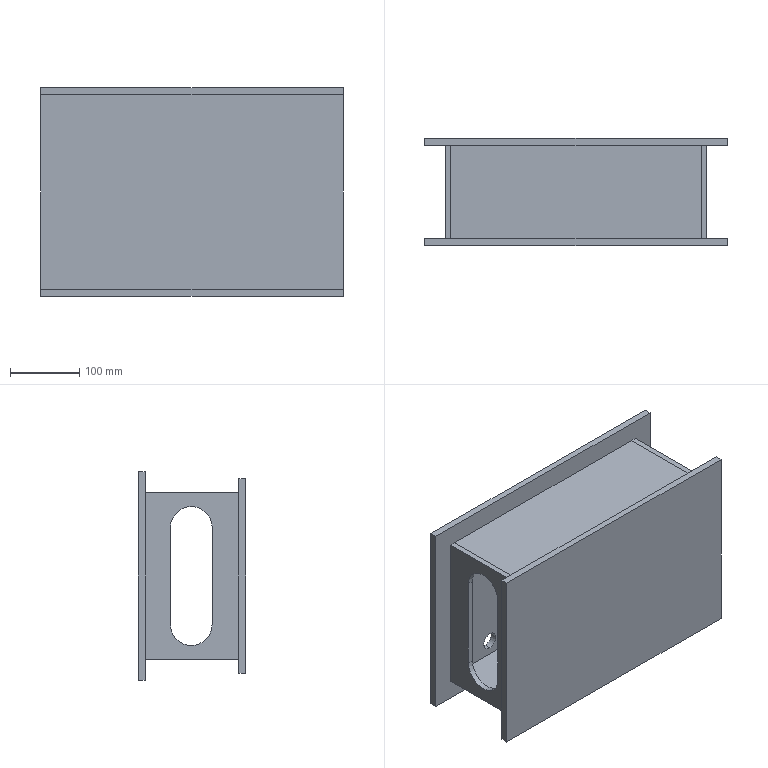Part | STEP file | Motor lower seat 2_Default<As machined> | 6 solids | 54 faces | box 436 x 154.533 x 300 mm | volume 3621040 mm3 | plane 40 | cylinder 14 | commonest cylinder face diameters 25 x8 60 x6